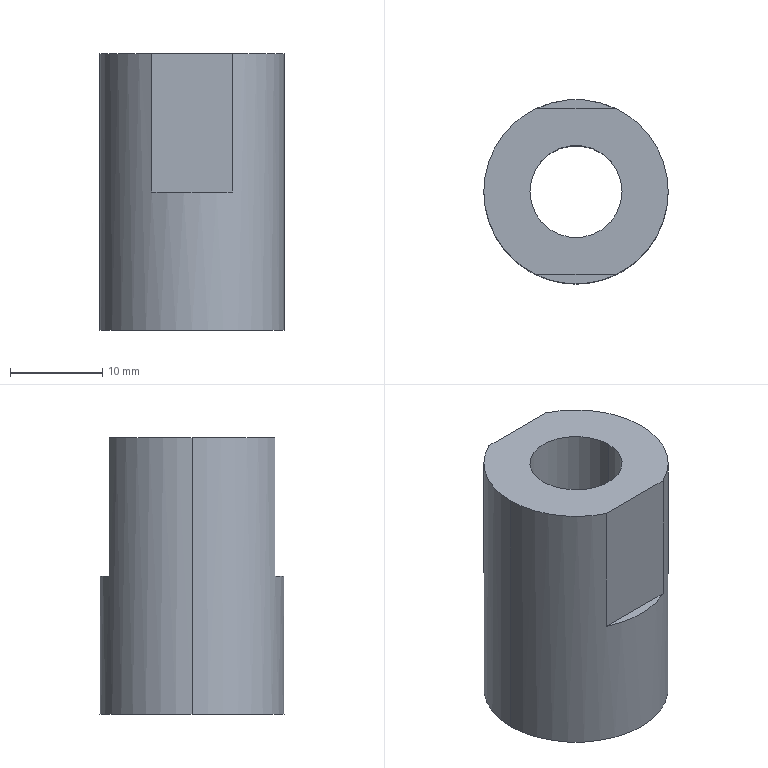Part | STEP file | Cylinder joint | 1 solid | 10 faces | box 20 x 20 x 30 mm | volume 6892 mm3 | plane 6 | cylinder 4 | commonest cylinder face diameters 10 x2 20 x2
STEP:
#1=CARTESIAN_POINT('',(0.,0.,0.));
#2=DIRECTION('',(0.,0.,1.));
#3=DIRECTION('',(1.,0.,0.));
#4=AXIS2_PLACEMENT_3D('',#1,#2,#3);
#5=CARTESIAN_POINT('',(4.359,9.,30.));
#6=VERTEX_POINT('',#5);
#7=CARTESIAN_POINT('',(10.,0.,30.));
#8=VERTEX_POINT('',#7);
#9=CARTESIAN_POINT('',(0.,0.,30.));
#10=DIRECTION('',(0.,0.,-1.));
#11=DIRECTION('',(-1.,0.,0.));
#12=AXIS2_PLACEMENT_3D('',#9,#10,#11);
#13=CIRCLE('',#12,10.);
#14=CARTESIAN_POINT('',(0.,0.,30.));
#15=DIRECTION('',(0.,0.,-1.));
#16=DIRECTION('',(-1.,0.,0.));
#17=AXIS2_PLACEMENT_3D('',#14,#15,#16);
#18=CYLINDRICAL_SURFACE('',#17,10.);
#19=CARTESIAN_POINT('',(0.,0.));
#20=DIRECTION('',(1.,0.));
#21=VECTOR('',#20,1.);
#22=LINE('',#19,#21);
#23=(GEOMETRIC_REPRESENTATION_CONTEXT(2)PARAMETRIC_REPRESENTATION_CONTEXT()REPRESENTATION_CONTEXT('',''));
#24=DEFINITIONAL_REPRESENTATION('',(#22),#23);
#25=PCURVE('',#18,#24);
#26=CARTESIAN_POINT('',(0.,0.,30.));
#27=DIRECTION('',(0.,0.,1.));
#28=DIRECTION('',(1.,0.,0.));
#29=AXIS2_PLACEMENT_3D('',#26,#27,#28);
#30=PLANE('',#29);
#31=CARTESIAN_POINT('',(-10.,0.));
#32=CARTESIAN_POINT('',(-10.,17.321));
#33=CARTESIAN_POINT('',(5.,8.66));
#34=CARTESIAN_POINT('',(20.,0.));
#35=CARTESIAN_POINT('',(5.,-8.66));
#36=CARTESIAN_POINT('',(-10.,-17.321));
#37=CARTESIAN_POINT('',(-10.,0.));
#38=(BOUNDED_CURVE()B_SPLINE_CURVE(2,(#31,#32,#33,#34,#35,#36,#37),.UNSPECIFIED.,.T.,.F.)B_SPLINE_CURVE_WITH_KNOTS((1,2,2,2,2,1),(-2.094,0.,2.094,4.189,6.283,8.378),.UNSPECIFIED.)CURVE()GEOMETRIC_REPRESENTATION_ITEM()RATIONAL_B_SPLINE_CURVE((1.,0.5,1.,0.5,1.,0.5,1.))REPRESENTATION_ITEM(''));
#39=(GEOMETRIC_REPRESENTATION_CONTEXT(2)PARAMETRIC_REPRESENTATION_CONTEXT()REPRESENTATION_CONTEXT('',''));
#40=DEFINITIONAL_REPRESENTATION('',(#38),#39);
#41=PCURVE('',#30,#40);
#42=SURFACE_CURVE('',#13,(#25,#41),.PCURVE_S1.);
#43=EDGE_CURVE('',#6,#8,#42,.T.);
#44=ORIENTED_EDGE('',*,*,#43,.T.);
#45=CARTESIAN_POINT('',(10.,0.,0.));
#46=VERTEX_POINT('',#45);
#47=CARTESIAN_POINT('',(10.,0.,30.));
#48=DIRECTION('',(0.,0.,-1.));
#49=VECTOR('',#48,1.);
#50=LINE('',#47,#49);
#51=CARTESIAN_POINT('',(3.142,0.));
#52=DIRECTION('',(0.,1.));
#53=VECTOR('',#52,1.);
#54=LINE('',#51,#53);
#55=(GEOMETRIC_REPRESENTATION_CONTEXT(2)PARAMETRIC_REPRESENTATION_CONTEXT()REPRESENTATION_CONTEXT('',''));
#56=DEFINITIONAL_REPRESENTATION('',(#54),#55);
#57=PCURVE('',#18,#56);
#58=CARTESIAN_POINT('',(0.,0.,30.));
#59=DIRECTION('',(0.,0.,-1.));
#60=DIRECTION('',(-1.,0.,0.));
#61=AXIS2_PLACEMENT_3D('',#58,#59,#60);
#62=CYLINDRICAL_SURFACE('',#61,10.);
#63=CARTESIAN_POINT('',(3.142,0.));
#64=DIRECTION('',(0.,1.));
#65=VECTOR('',#64,1.);
#66=LINE('',#63,#65);
#67=(GEOMETRIC_REPRESENTATION_CONTEXT(2)PARAMETRIC_REPRESENTATION_CONTEXT()REPRESENTATION_CONTEXT('',''));
#68=DEFINITIONAL_REPRESENTATION('',(#66),#67);
#69=PCURVE('',#62,#68);
#70=SURFACE_CURVE('',#50,(#57,#69),.PCURVE_S1.);
#71=EDGE_CURVE('',#8,#46,#70,.T.);
#72=ORIENTED_EDGE('',*,*,#71,.T.);
#73=CARTESIAN_POINT('',(-10.,0.,0.));
#74=VERTEX_POINT('',#73);
#75=CARTESIAN_POINT('',(0.,0.,0.));
#76=DIRECTION('',(0.,0.,1.));
#77=DIRECTION('',(-1.,0.,0.));
#78=AXIS2_PLACEMENT_3D('',#75,#76,#77);
#79=CIRCLE('',#78,10.);
#80=CARTESIAN_POINT('',(6.283,30.));
#81=DIRECTION('',(-1.,0.));
#82=VECTOR('',#81,1.);
#83=LINE('',#80,#82);
#84=(GEOMETRIC_REPRESENTATION_CONTEXT(2)PARAMETRIC_REPRESENTATION_CONTEXT()REPRESENTATION_CONTEXT('',''));
#85=DEFINITIONAL_REPRESENTATION('',(#83),#84);
#86=PCURVE('',#18,#85);
#87=CARTESIAN_POINT('',(0.,0.,0.));
#88=DIRECTION('',(0.,0.,1.));
#89=DIRECTION('',(1.,0.,0.));
#90=AXIS2_PLACEMENT_3D('',#87,#88,#89);
#91=PLANE('',#90);
#92=CARTESIAN_POINT('',(0.,0.));
#93=DIRECTION('',(-1.,0.));
#94=AXIS2_PLACEMENT_2D('',#92,#93);
#95=CIRCLE('',#94,10.);
#96=(GEOMETRIC_REPRESENTATION_CONTEXT(2)PARAMETRIC_REPRESENTATION_CONTEXT()REPRESENTATION_CONTEXT('',''));
#97=DEFINITIONAL_REPRESENTATION('',(#95),#96);
#98=PCURVE('',#91,#97);
#99=SURFACE_CURVE('',#79,(#86,#98),.PCURVE_S1.);
#100=EDGE_CURVE('',#46,#74,#99,.T.);
#101=ORIENTED_EDGE('',*,*,#100,.T.);
#102=CARTESIAN_POINT('',(-10.,0.,30.));
#103=VERTEX_POINT('',#102);
#104=CARTESIAN_POINT('',(-10.,0.,30.));
#105=DIRECTION('',(0.,0.,-1.));
#106=VECTOR('',#105,1.);
#107=LINE('',#104,#106);
#108=CARTESIAN_POINT('',(0.,0.));
#109=DIRECTION('',(0.,1.));
#110=VECTOR('',#109,1.);
#111=LINE('',#108,#110);
#112=(GEOMETRIC_REPRESENTATION_CONTEXT(2)PARAMETRIC_REPRESENTATION_CONTEXT()REPRESENTATION_CONTEXT('',''));
#113=DEFINITIONAL_REPRESENTATION('',(#111),#112);
#114=PCURVE('',#18,#113);
#115=CARTESIAN_POINT('',(6.283,0.));
#116=DIRECTION('',(0.,1.));
#117=VECTOR('',#116,1.);
#118=LINE('',#115,#117);
#119=(GEOMETRIC_REPRESENTATION_CONTEXT(2)PARAMETRIC_REPRESENTATION_CONTEXT()REPRESENTATION_CONTEXT('',''));
#120=DEFINITIONAL_REPRESENTATION('',(#118),#119);
#121=PCURVE('',#62,#120);
#122=SURFACE_CURVE('',#107,(#114,#121),.PCURVE_S1.);
#123=EDGE_CURVE('',#103,#74,#122,.T.);
#124=ORIENTED_EDGE('',*,*,#123,.F.);
#125=CARTESIAN_POINT('',(-4.359,9.,30.));
#126=VERTEX_POINT('',#125);
#127=CARTESIAN_POINT('',(0.,0.,30.));
#128=DIRECTION('',(0.,0.,-1.));
#129=DIRECTION('',(-1.,0.,0.));
#130=AXIS2_PLACEMENT_3D('',#127,#128,#129);
#131=CIRCLE('',#130,10.);
#132=CARTESIAN_POINT('',(0.,0.));
#133=DIRECTION('',(1.,0.));
#134=VECTOR('',#133,1.);
#135=LINE('',#132,#134);
#136=(GEOMETRIC_REPRESENTATION_CONTEXT(2)PARAMETRIC_REPRESENTATION_CONTEXT()REPRESENTATION_CONTEXT('',''));
#137=DEFINITIONAL_REPRESENTATION('',(#135),#136);
#138=PCURVE('',#18,#137);
#139=CARTESIAN_POINT('',(-10.,0.));
#140=CARTESIAN_POINT('',(-10.,17.321));
#141=CARTESIAN_POINT('',(5.,8.66));
#142=CARTESIAN_POINT('',(20.,0.));
#143=CARTESIAN_POINT('',(5.,-8.66));
#144=CARTESIAN_POINT('',(-10.,-17.321));
#145=CARTESIAN_POINT('',(-10.,0.));
#146=(BOUNDED_CURVE()B_SPLINE_CURVE(2,(#139,#140,#141,#142,#143,#144,#145),.UNSPECIFIED.,.T.,.F.)B_SPLINE_CURVE_WITH_KNOTS((1,2,2,2,2,1),(-2.094,0.,2.094,4.189,6.283,8.378),.UNSPECIFIED.)CURVE()GEOMETRIC_REPRESENTATION_ITEM()RATIONAL_B_SPLINE_CURVE((1.,0.5,1.,0.5,1.,0.5,1.))REPRESENTATION_ITEM(''));
#147=(GEOMETRIC_REPRESENTATION_CONTEXT(2)PARAMETRIC_REPRESENTATION_CONTEXT()REPRESENTATION_CONTEXT('',''));
#148=DEFINITIONAL_REPRESENTATION('',(#146),#147);
#149=PCURVE('',#30,#148);
#150=SURFACE_CURVE('',#131,(#138,#149),.PCURVE_S1.);
#151=EDGE_CURVE('',#103,#126,#150,.T.);
#152=ORIENTED_EDGE('',*,*,#151,.T.);
#153=CARTESIAN_POINT('',(-4.359,9.,15.));
#154=VERTEX_POINT('',#153);
#155=CARTESIAN_POINT('',(-4.359,9.,30.));
#156=DIRECTION('',(0.,0.,-1.));
#157=VECTOR('',#156,1.);
#158=LINE('',#155,#157);
#159=CARTESIAN_POINT('',(1.12,0.));
#160=DIRECTION('',(0.,1.));
#161=VECTOR('',#160,1.);
#162=LINE('',#159,#161);
#163=(GEOMETRIC_REPRESENTATION_CONTEXT(2)PARAMETRIC_REPRESENTATION_CONTEXT()REPRESENTATION_CONTEXT('',''));
#164=DEFINITIONAL_REPRESENTATION('',(#162),#163);
#165=PCURVE('',#18,#164);
#166=CARTESIAN_POINT('',(-4.359,9.,15.));
#167=DIRECTION('',(0.,-1.,0.));
#168=DIRECTION('',(0.,0.,-1.));
#169=AXIS2_PLACEMENT_3D('',#166,#167,#168);
#170=PLANE('',#169);
#171=CARTESIAN_POINT('',(-15.,0.));
#172=DIRECTION('',(1.,0.));
#173=VECTOR('',#172,1.);
#174=LINE('',#171,#173);
#175=(GEOMETRIC_REPRESENTATION_CONTEXT(2)PARAMETRIC_REPRESENTATION_CONTEXT()REPRESENTATION_CONTEXT('',''));
#176=DEFINITIONAL_REPRESENTATION('',(#174),#175);
#177=PCURVE('',#170,#176);
#178=SURFACE_CURVE('',#158,(#165,#177),.PCURVE_S1.);
#179=EDGE_CURVE('',#126,#154,#178,.T.);
#180=ORIENTED_EDGE('',*,*,#179,.T.);
#181=CARTESIAN_POINT('',(4.359,9.,15.));
#182=VERTEX_POINT('',#181);
#183=CARTESIAN_POINT('',(0.,0.,15.));
#184=DIRECTION('',(0.,0.,-1.));
#185=DIRECTION('',(-1.,0.,0.));
#186=AXIS2_PLACEMENT_3D('',#183,#184,#185);
#187=CIRCLE('',#186,10.);
#188=CARTESIAN_POINT('',(0.,15.));
#189=DIRECTION('',(1.,0.));
#190=VECTOR('',#189,1.);
#191=LINE('',#188,#190);
#192=(GEOMETRIC_REPRESENTATION_CONTEXT(2)PARAMETRIC_REPRESENTATION_CONTEXT()REPRESENTATION_CONTEXT('',''));
#193=DEFINITIONAL_REPRESENTATION('',(#191),#192);
#194=PCURVE('',#18,#193);
#195=CARTESIAN_POINT('',(0.,0.,15.));
#196=DIRECTION('',(0.,0.,1.));
#197=DIRECTION('',(1.,0.,0.));
#198=AXIS2_PLACEMENT_3D('',#195,#196,#197);
#199=PLANE('',#198);
#200=CARTESIAN_POINT('',(-10.,0.));
#201=CARTESIAN_POINT('',(-10.,17.321));
#202=CARTESIAN_POINT('',(5.,8.66));
#203=CARTESIAN_POINT('',(20.,0.));
#204=CARTESIAN_POINT('',(5.,-8.66));
#205=CARTESIAN_POINT('',(-10.,-17.321));
#206=CARTESIAN_POINT('',(-10.,0.));
#207=(BOUNDED_CURVE()B_SPLINE_CURVE(2,(#200,#201,#202,#203,#204,#205,#206),.UNSPECIFIED.,.T.,.F.)B_SPLINE_CURVE_WITH_KNOTS((1,2,2,2,2,1),(-2.094,0.,2.094,4.189,6.283,8.378),.UNSPECIFIED.)CURVE()GEOMETRIC_REPRESENTATION_ITEM()RATIONAL_B_SPLINE_CURVE((1.,0.5,1.,0.5,1.,0.5,1.))REPRESENTATION_ITEM(''));
#208=(GEOMETRIC_REPRESENTATION_CONTEXT(2)PARAMETRIC_REPRESENTATION_CONTEXT()REPRESENTATION_CONTEXT('',''));
#209=DEFINITIONAL_REPRESENTATION('',(#207),#208);
#210=PCURVE('',#199,#209);
#211=SURFACE_CURVE('',#187,(#194,#210),.PCURVE_S1.);
#212=EDGE_CURVE('',#154,#182,#211,.T.);
#213=ORIENTED_EDGE('',*,*,#212,.T.);
#214=CARTESIAN_POINT('',(4.359,9.,30.));
#215=DIRECTION('',(0.,0.,1.));
#216=VECTOR('',#215,1.);
#217=LINE('',#214,#216);
#218=CARTESIAN_POINT('',(2.022,0.));
#219=DIRECTION('',(0.,-1.));
#220=VECTOR('',#219,1.);
#221=LINE('',#218,#220);
#222=(GEOMETRIC_REPRESENTATION_CONTEXT(2)PARAMETRIC_REPRESENTATION_CONTEXT()REPRESENTATION_CONTEXT('',''));
#223=DEFINITIONAL_REPRESENTATION('',(#221),#222);
#224=PCURVE('',#18,#223);
#225=CARTESIAN_POINT('',(-15.,8.718));
#226=DIRECTION('',(-1.,0.));
#227=VECTOR('',#226,1.);
#228=LINE('',#225,#227);
#229=(GEOMETRIC_REPRESENTATION_CONTEXT(2)PARAMETRIC_REPRESENTATION_CONTEXT()REPRESENTATION_CONTEXT('',''));
#230=DEFINITIONAL_REPRESENTATION('',(#228),#229);
#231=PCURVE('',#170,#230);
#232=SURFACE_CURVE('',#217,(#224,#231),.PCURVE_S1.);
#233=EDGE_CURVE('',#182,#6,#232,.T.);
#234=ORIENTED_EDGE('',*,*,#233,.T.);
#235=EDGE_LOOP('',(#44,#72,#101,#124,#152,#180,#213,#234));
#236=FACE_BOUND('',#235,.T.);
#237=ADVANCED_FACE('',(#236),#18,.T.);
#238=CARTESIAN_POINT('',(-5.,0.,30.));
#239=VERTEX_POINT('',#238);
#240=CARTESIAN_POINT('',(-5.,0.,0.));
#241=VERTEX_POINT('',#240);
#242=CARTESIAN_POINT('',(-5.,0.,30.));
#243=DIRECTION('',(0.,0.,-1.));
#244=VECTOR('',#243,1.);
#245=LINE('',#242,#244);
#246=CARTESIAN_POINT('',(0.,0.,30.));
#247=DIRECTION('',(0.,0.,-1.));
#248=DIRECTION('',(-1.,0.,0.));
#249=AXIS2_PLACEMENT_3D('',#246,#247,#248);
#250=CYLINDRICAL_SURFACE('',#249,5.);
#251=CARTESIAN_POINT('',(6.283,0.));
#252=DIRECTION('',(0.,1.));
#253=VECTOR('',#252,1.);
#254=LINE('',#251,#253);
#255=(GEOMETRIC_REPRESENTATION_CONTEXT(2)PARAMETRIC_REPRESENTATION_CONTEXT()REPRESENTATION_CONTEXT('',''));
#256=DEFINITIONAL_REPRESENTATION('',(#254),#255);
#257=PCURVE('',#250,#256);
#258=CARTESIAN_POINT('',(0.,0.,30.));
#259=DIRECTION('',(0.,0.,-1.));
#260=DIRECTION('',(-1.,0.,0.));
#261=AXIS2_PLACEMENT_3D('',#258,#259,#260);
#262=CYLINDRICAL_SURFACE('',#261,5.);
#263=CARTESIAN_POINT('',(0.,0.));
#264=DIRECTION('',(0.,1.));
#265=VECTOR('',#264,1.);
#266=LINE('',#263,#265);
#267=(GEOMETRIC_REPRESENTATION_CONTEXT(2)PARAMETRIC_REPRESENTATION_CONTEXT()REPRESENTATION_CONTEXT('',''));
#268=DEFINITIONAL_REPRESENTATION('',(#266),#267);
#269=PCURVE('',#262,#268);
#270=SURFACE_CURVE('',#245,(#257,#269),.PCURVE_S1.);
#271=EDGE_CURVE('',#239,#241,#270,.T.);
#272=ORIENTED_EDGE('',*,*,#271,.T.);
#273=CARTESIAN_POINT('',(5.,0.,0.));
#274=VERTEX_POINT('',#273);
#275=CARTESIAN_POINT('',(0.,0.,0.));
#276=DIRECTION('',(0.,0.,-1.));
#277=DIRECTION('',(-1.,0.,0.));
#278=AXIS2_PLACEMENT_3D('',#275,#276,#277);
#279=CIRCLE('',#278,5.);
#280=CARTESIAN_POINT('',(0.,30.));
#281=DIRECTION('',(1.,0.));
#282=VECTOR('',#281,1.);
#283=LINE('',#280,#282);
#284=(GEOMETRIC_REPRESENTATION_CONTEXT(2)PARAMETRIC_REPRESENTATION_CONTEXT()REPRESENTATION_CONTEXT('',''));
#285=DEFINITIONAL_REPRESENTATION('',(#283),#284);
#286=PCURVE('',#250,#285);
#287=CARTESIAN_POINT('',(-5.,0.));
#288=CARTESIAN_POINT('',(-5.,8.66));
#289=CARTESIAN_POINT('',(2.5,4.33));
#290=CARTESIAN_POINT('',(10.,0.));
#291=CARTESIAN_POINT('',(2.5,-4.33));
#292=CARTESIAN_POINT('',(-5.,-8.66));
#293=CARTESIAN_POINT('',(-5.,0.));
#294=(BOUNDED_CURVE()B_SPLINE_CURVE(2,(#287,#288,#289,#290,#291,#292,#293),.UNSPECIFIED.,.T.,.F.)B_SPLINE_CURVE_WITH_KNOTS((1,2,2,2,2,1),(-2.094,0.,2.094,4.189,6.283,8.378),.UNSPECIFIED.)CURVE()GEOMETRIC_REPRESENTATION_ITEM()RATIONAL_B_SPLINE_CURVE((1.,0.5,1.,0.5,1.,0.5,1.))REPRESENTATION_ITEM(''));
#295=(GEOMETRIC_REPRESENTATION_CONTEXT(2)PARAMETRIC_REPRESENTATION_CONTEXT()REPRESENTATION_CONTEXT('',''));
#296=DEFINITIONAL_REPRESENTATION('',(#294),#295);
#297=PCURVE('',#91,#296);
#298=SURFACE_CURVE('',#279,(#286,#297),.PCURVE_S1.);
#299=EDGE_CURVE('',#274,#241,#298,.T.);
#300=ORIENTED_EDGE('',*,*,#299,.F.);
#301=CARTESIAN_POINT('',(5.,0.,30.));
#302=VERTEX_POINT('',#301);
#303=CARTESIAN_POINT('',(5.,0.,30.));
#304=DIRECTION('',(0.,0.,-1.));
#305=VECTOR('',#304,1.);
#306=LINE('',#303,#305);
#307=CARTESIAN_POINT('',(3.142,0.));
#308=DIRECTION('',(0.,1.));
#309=VECTOR('',#308,1.);
#310=LINE('',#307,#309);
#311=(GEOMETRIC_REPRESENTATION_CONTEXT(2)PARAMETRIC_REPRESENTATION_CONTEXT()REPRESENTATION_CONTEXT('',''));
#312=DEFINITIONAL_REPRESENTATION('',(#310),#311);
#313=PCURVE('',#250,#312);
#314=CARTESIAN_POINT('',(3.142,0.));
#315=DIRECTION('',(0.,1.));
#316=VECTOR('',#315,1.);
#317=LINE('',#314,#316);
#318=(GEOMETRIC_REPRESENTATION_CONTEXT(2)PARAMETRIC_REPRESENTATION_CONTEXT()REPRESENTATION_CONTEXT('',''));
#319=DEFINITIONAL_REPRESENTATION('',(#317),#318);
#320=PCURVE('',#262,#319);
#321=SURFACE_CURVE('',#306,(#313,#320),.PCURVE_S1.);
#322=EDGE_CURVE('',#302,#274,#321,.T.);
#323=ORIENTED_EDGE('',*,*,#322,.F.);
#324=CARTESIAN_POINT('',(0.,0.,30.));
#325=DIRECTION('',(0.,0.,-1.));
#326=DIRECTION('',(-1.,0.,0.));
#327=AXIS2_PLACEMENT_3D('',#324,#325,#326);
#328=CIRCLE('',#327,5.);
#329=CARTESIAN_POINT('',(0.,0.));
#330=DIRECTION('',(1.,0.));
#331=VECTOR('',#330,1.);
#332=LINE('',#329,#331);
#333=(GEOMETRIC_REPRESENTATION_CONTEXT(2)PARAMETRIC_REPRESENTATION_CONTEXT()REPRESENTATION_CONTEXT('',''));
#334=DEFINITIONAL_REPRESENTATION('',(#332),#333);
#335=PCURVE('',#250,#334);
#336=CARTESIAN_POINT('',(-5.,0.));
#337=CARTESIAN_POINT('',(-5.,8.66));
#338=CARTESIAN_POINT('',(2.5,4.33));
#339=CARTESIAN_POINT('',(10.,0.));
#340=CARTESIAN_POINT('',(2.5,-4.33));
#341=CARTESIAN_POINT('',(-5.,-8.66));
#342=CARTESIAN_POINT('',(-5.,0.));
#343=(BOUNDED_CURVE()B_SPLINE_CURVE(2,(#336,#337,#338,#339,#340,#341,#342),.UNSPECIFIED.,.T.,.F.)B_SPLINE_CURVE_WITH_KNOTS((1,2,2,2,2,1),(-2.094,0.,2.094,4.189,6.283,8.378),.UNSPECIFIED.)CURVE()GEOMETRIC_REPRESENTATION_ITEM()RATIONAL_B_SPLINE_CURVE((1.,0.5,1.,0.5,1.,0.5,1.))REPRESENTATION_ITEM(''));
#344=(GEOMETRIC_REPRESENTATION_CONTEXT(2)PARAMETRIC_REPRESENTATION_CONTEXT()REPRESENTATION_CONTEXT('',''));
#345=DEFINITIONAL_REPRESENTATION('',(#343),#344);
#346=PCURVE('',#30,#345);
#347=SURFACE_CURVE('',#328,(#335,#346),.PCURVE_S1.);
#348=EDGE_CURVE('',#302,#239,#347,.T.);
#349=ORIENTED_EDGE('',*,*,#348,.T.);
#350=EDGE_LOOP('',(#272,#300,#323,#349));
#351=FACE_BOUND('',#350,.F.);
#352=ADVANCED_FACE('',(#351),#250,.F.);
#353=ORIENTED_EDGE('',*,*,#71,.F.);
#354=CARTESIAN_POINT('',(4.359,-9.,30.));
#355=VERTEX_POINT('',#354);
#356=CARTESIAN_POINT('',(0.,0.,30.));
#357=DIRECTION('',(0.,0.,-1.));
#358=DIRECTION('',(-1.,0.,0.));
#359=AXIS2_PLACEMENT_3D('',#356,#357,#358);
#360=CIRCLE('',#359,10.);
#361=CARTESIAN_POINT('',(0.,0.));
#362=DIRECTION('',(1.,0.));
#363=VECTOR('',#362,1.);
#364=LINE('',#361,#363);
#365=(GEOMETRIC_REPRESENTATION_CONTEXT(2)PARAMETRIC_REPRESENTATION_CONTEXT()REPRESENTATION_CONTEXT('',''));
#366=DEFINITIONAL_REPRESENTATION('',(#364),#365);
#367=PCURVE('',#62,#366);
#368=CARTESIAN_POINT('',(-10.,0.));
#369=CARTESIAN_POINT('',(-10.,17.321));
#370=CARTESIAN_POINT('',(5.,8.66));
#371=CARTESIAN_POINT('',(20.,0.));
#372=CARTESIAN_POINT('',(5.,-8.66));
#373=CARTESIAN_POINT('',(-10.,-17.321));
#374=CARTESIAN_POINT('',(-10.,0.));
#375=(BOUNDED_CURVE()B_SPLINE_CURVE(2,(#368,#369,#370,#371,#372,#373,#374),.UNSPECIFIED.,.T.,.F.)B_SPLINE_CURVE_WITH_KNOTS((1,2,2,2,2,1),(-2.094,0.,2.094,4.189,6.283,8.378),.UNSPECIFIED.)CURVE()GEOMETRIC_REPRESENTATION_ITEM()RATIONAL_B_SPLINE_CURVE((1.,0.5,1.,0.5,1.,0.5,1.))REPRESENTATION_ITEM(''));
#376=(GEOMETRIC_REPRESENTATION_CONTEXT(2)PARAMETRIC_REPRESENTATION_CONTEXT()REPRESENTATION_CONTEXT('',''));
#377=DEFINITIONAL_REPRESENTATION('',(#375),#376);
#378=PCURVE('',#30,#377);
#379=SURFACE_CURVE('',#360,(#367,#378),.PCURVE_S1.);
#380=EDGE_CURVE('',#8,#355,#379,.T.);
#381=ORIENTED_EDGE('',*,*,#380,.T.);
#382=CARTESIAN_POINT('',(4.359,-9.,15.));
#383=VERTEX_POINT('',#382);
#384=CARTESIAN_POINT('',(4.359,-9.,30.));
#385=DIRECTION('',(0.,0.,-1.));
#386=VECTOR('',#385,1.);
#387=LINE('',#384,#386);
#388=CARTESIAN_POINT('',(4.261,0.));
#389=DIRECTION('',(0.,1.));
#390=VECTOR('',#389,1.);
#391=LINE('',#388,#390);
#392=(GEOMETRIC_REPRESENTATION_CONTEXT(2)PARAMETRIC_REPRESENTATION_CONTEXT()REPRESENTATION_CONTEXT('',''));
#393=DEFINITIONAL_REPRESENTATION('',(#391),#392);
#394=PCURVE('',#62,#393);
#395=CARTESIAN_POINT('',(-4.359,-9.,15.));
#396=DIRECTION('',(0.,1.,0.));
#397=DIRECTION('',(0.,0.,1.));
#398=AXIS2_PLACEMENT_3D('',#395,#396,#397);
#399=PLANE('',#398);
#400=CARTESIAN_POINT('',(15.,8.718));
#401=DIRECTION('',(-1.,0.));
#402=VECTOR('',#401,1.);
#403=LINE('',#400,#402);
#404=(GEOMETRIC_REPRESENTATION_CONTEXT(2)PARAMETRIC_REPRESENTATION_CONTEXT()REPRESENTATION_CONTEXT('',''));
#405=DEFINITIONAL_REPRESENTATION('',(#403),#404);
#406=PCURVE('',#399,#405);
#407=SURFACE_CURVE('',#387,(#394,#406),.PCURVE_S1.);
#408=EDGE_CURVE('',#355,#383,#407,.T.);
#409=ORIENTED_EDGE('',*,*,#408,.T.);
#410=CARTESIAN_POINT('',(-4.359,-9.,15.));
#411=VERTEX_POINT('',#410);
#412=CARTESIAN_POINT('',(0.,0.,15.));
#413=DIRECTION('',(0.,0.,-1.));
#414=DIRECTION('',(-1.,0.,0.));
#415=AXIS2_PLACEMENT_3D('',#412,#413,#414);
#416=CIRCLE('',#415,10.);
#417=CARTESIAN_POINT('',(0.,15.));
#418=DIRECTION('',(1.,0.));
#419=VECTOR('',#418,1.);
#420=LINE('',#417,#419);
#421=(GEOMETRIC_REPRESENTATION_CONTEXT(2)PARAMETRIC_REPRESENTATION_CONTEXT()REPRESENTATION_CONTEXT('',''));
#422=DEFINITIONAL_REPRESENTATION('',(#420),#421);
#423=PCURVE('',#62,#422);
#424=CARTESIAN_POINT('',(0.,0.,15.));
#425=DIRECTION('',(0.,0.,1.));
#426=DIRECTION('',(1.,0.,0.));
#427=AXIS2_PLACEMENT_3D('',#424,#425,#426);
#428=PLANE('',#427);
#429=CARTESIAN_POINT('',(-10.,0.));
#430=CARTESIAN_POINT('',(-10.,17.321));
#431=CARTESIAN_POINT('',(5.,8.66));
#432=CARTESIAN_POINT('',(20.,0.));
#433=CARTESIAN_POINT('',(5.,-8.66));
#434=CARTESIAN_POINT('',(-10.,-17.321));
#435=CARTESIAN_POINT('',(-10.,0.));
#436=(BOUNDED_CURVE()B_SPLINE_CURVE(2,(#429,#430,#431,#432,#433,#434,#435),.UNSPECIFIED.,.T.,.F.)B_SPLINE_CURVE_WITH_KNOTS((1,2,2,2,2,1),(-2.094,0.,2.094,4.189,6.283,8.378),.UNSPECIFIED.)CURVE()GEOMETRIC_REPRESENTATION_ITEM()RATIONAL_B_SPLINE_CURVE((1.,0.5,1.,0.5,1.,0.5,1.))REPRESENTATION_ITEM(''));
#437=(GEOMETRIC_REPRESENTATION_CONTEXT(2)PARAMETRIC_REPRESENTATION_CONTEXT()REPRESENTATION_CONTEXT('',''));
#438=DEFINITIONAL_REPRESENTATION('',(#436),#437);
#439=PCURVE('',#428,#438);
#440=SURFACE_CURVE('',#416,(#423,#439),.PCURVE_S1.);
#441=EDGE_CURVE('',#383,#411,#440,.T.);
#442=ORIENTED_EDGE('',*,*,#441,.T.);
#443=CARTESIAN_POINT('',(-4.359,-9.,30.));
#444=VERTEX_POINT('',#443);
#445=CARTESIAN_POINT('',(-4.359,-9.,30.));
#446=DIRECTION('',(0.,0.,1.));
#447=VECTOR('',#446,1.);
#448=LINE('',#445,#447);
#449=CARTESIAN_POINT('',(5.163,0.));
#450=DIRECTION('',(0.,-1.));
#451=VECTOR('',#450,1.);
#452=LINE('',#449,#451);
#453=(GEOMETRIC_REPRESENTATION_CONTEXT(2)PARAMETRIC_REPRESENTATION_CONTEXT()REPRESENTATION_CONTEXT('',''));
#454=DEFINITIONAL_REPRESENTATION('',(#452),#453);
#455=PCURVE('',#62,#454);
#456=CARTESIAN_POINT('',(15.,0.));
#457=DIRECTION('',(1.,0.));
#458=VECTOR('',#457,1.);
#459=LINE('',#456,#458);
#460=(GEOMETRIC_REPRESENTATION_CONTEXT(2)PARAMETRIC_REPRESENTATION_CONTEXT()REPRESENTATION_CONTEXT('',''));
#461=DEFINITIONAL_REPRESENTATION('',(#459),#460);
#462=PCURVE('',#399,#461);
#463=SURFACE_CURVE('',#448,(#455,#462),.PCURVE_S1.);
#464=EDGE_CURVE('',#411,#444,#463,.T.);
#465=ORIENTED_EDGE('',*,*,#464,.T.);
#466=CARTESIAN_POINT('',(0.,0.,30.));
#467=DIRECTION('',(0.,0.,-1.));
#468=DIRECTION('',(-1.,0.,0.));
#469=AXIS2_PLACEMENT_3D('',#466,#467,#468);
#470=CIRCLE('',#469,10.);
#471=CARTESIAN_POINT('',(0.,0.));
#472=DIRECTION('',(1.,0.));
#473=VECTOR('',#472,1.);
#474=LINE('',#471,#473);
#475=(GEOMETRIC_REPRESENTATION_CONTEXT(2)PARAMETRIC_REPRESENTATION_CONTEXT()REPRESENTATION_CONTEXT('',''));
#476=DEFINITIONAL_REPRESENTATION('',(#474),#475);
#477=PCURVE('',#62,#476);
#478=CARTESIAN_POINT('',(-10.,0.));
#479=CARTESIAN_POINT('',(-10.,17.321));
#480=CARTESIAN_POINT('',(5.,8.66));
#481=CARTESIAN_POINT('',(20.,0.));
#482=CARTESIAN_POINT('',(5.,-8.66));
#483=CARTESIAN_POINT('',(-10.,-17.321));
#484=CARTESIAN_POINT('',(-10.,0.));
#485=(BOUNDED_CURVE()B_SPLINE_CURVE(2,(#478,#479,#480,#481,#482,#483,#484),.UNSPECIFIED.,.T.,.F.)B_SPLINE_CURVE_WITH_KNOTS((1,2,2,2,2,1),(-2.094,0.,2.094,4.189,6.283,8.378),.UNSPECIFIED.)CURVE()GEOMETRIC_REPRESENTATION_ITEM()RATIONAL_B_SPLINE_CURVE((1.,0.5,1.,0.5,1.,0.5,1.))REPRESENTATION_ITEM(''));
#486=(GEOMETRIC_REPRESENTATION_CONTEXT(2)PARAMETRIC_REPRESENTATION_CONTEXT()REPRESENTATION_CONTEXT('',''));
#487=DEFINITIONAL_REPRESENTATION('',(#485),#486);
#488=PCURVE('',#30,#487);
#489=SURFACE_CURVE('',#470,(#477,#488),.PCURVE_S1.);
#490=EDGE_CURVE('',#444,#103,#489,.T.);
#491=ORIENTED_EDGE('',*,*,#490,.T.);
#492=ORIENTED_EDGE('',*,*,#123,.T.);
#493=CARTESIAN_POINT('',(0.,0.,0.));
#494=DIRECTION('',(0.,0.,1.));
#495=DIRECTION('',(-1.,0.,0.));
#496=AXIS2_PLACEMENT_3D('',#493,#494,#495);
#497=CIRCLE('',#496,10.);
#498=CARTESIAN_POINT('',(6.283,30.));
#499=DIRECTION('',(-1.,0.));
#500=VECTOR('',#499,1.);
#501=LINE('',#498,#500);
#502=(GEOMETRIC_REPRESENTATION_CONTEXT(2)PARAMETRIC_REPRESENTATION_CONTEXT()REPRESENTATION_CONTEXT('',''));
#503=DEFINITIONAL_REPRESENTATION('',(#501),#502);
#504=PCURVE('',#62,#503);
#505=CARTESIAN_POINT('',(0.,0.));
#506=DIRECTION('',(-1.,0.));
#507=AXIS2_PLACEMENT_2D('',#505,#506);
#508=CIRCLE('',#507,10.);
#509=(GEOMETRIC_REPRESENTATION_CONTEXT(2)PARAMETRIC_REPRESENTATION_CONTEXT()REPRESENTATION_CONTEXT('',''));
#510=DEFINITIONAL_REPRESENTATION('',(#508),#509);
#511=PCURVE('',#91,#510);
#512=SURFACE_CURVE('',#497,(#504,#511),.PCURVE_S1.);
#513=EDGE_CURVE('',#74,#46,#512,.T.);
#514=ORIENTED_EDGE('',*,*,#513,.T.);
#515=EDGE_LOOP('',(#353,#381,#409,#442,#465,#491,#492,#514));
#516=FACE_BOUND('',#515,.T.);
#517=ADVANCED_FACE('',(#516),#62,.T.);
#518=ORIENTED_EDGE('',*,*,#233,.F.);
#519=CARTESIAN_POINT('',(-4.359,9.,15.));
#520=DIRECTION('',(1.,0.,0.));
#521=VECTOR('',#520,1.);
#522=LINE('',#519,#521);
#523=CARTESIAN_POINT('',(0.,0.));
#524=DIRECTION('',(0.,1.));
#525=VECTOR('',#524,1.);
#526=LINE('',#523,#525);
#527=(GEOMETRIC_REPRESENTATION_CONTEXT(2)PARAMETRIC_REPRESENTATION_CONTEXT()REPRESENTATION_CONTEXT('',''));
#528=DEFINITIONAL_REPRESENTATION('',(#526),#527);
#529=PCURVE('',#170,#528);
#530=CARTESIAN_POINT('',(-4.359,9.));
#531=DIRECTION('',(1.,0.));
#532=VECTOR('',#531,1.);
#533=LINE('',#530,#532);
#534=(GEOMETRIC_REPRESENTATION_CONTEXT(2)PARAMETRIC_REPRESENTATION_CONTEXT()REPRESENTATION_CONTEXT('',''));
#535=DEFINITIONAL_REPRESENTATION('',(#533),#534);
#536=PCURVE('',#199,#535);
#537=SURFACE_CURVE('',#522,(#529,#536),.PCURVE_S1.);
#538=EDGE_CURVE('',#154,#182,#537,.T.);
#539=ORIENTED_EDGE('',*,*,#538,.F.);
#540=ORIENTED_EDGE('',*,*,#179,.F.);
#541=CARTESIAN_POINT('',(-4.359,9.,30.));
#542=DIRECTION('',(-1.,0.,0.));
#543=VECTOR('',#542,1.);
#544=LINE('',#541,#543);
#545=CARTESIAN_POINT('',(-15.,0.));
#546=DIRECTION('',(0.,-1.));
#547=VECTOR('',#546,1.);
#548=LINE('',#545,#547);
#549=(GEOMETRIC_REPRESENTATION_CONTEXT(2)PARAMETRIC_REPRESENTATION_CONTEXT()REPRESENTATION_CONTEXT('',''));
#550=DEFINITIONAL_REPRESENTATION('',(#548),#549);
#551=PCURVE('',#170,#550);
#552=CARTESIAN_POINT('',(-4.359,9.));
#553=DIRECTION('',(-1.,0.));
#554=VECTOR('',#553,1.);
#555=LINE('',#552,#554);
#556=(GEOMETRIC_REPRESENTATION_CONTEXT(2)PARAMETRIC_REPRESENTATION_CONTEXT()REPRESENTATION_CONTEXT('',''));
#557=DEFINITIONAL_REPRESENTATION('',(#555),#556);
#558=PCURVE('',#30,#557);
#559=SURFACE_CURVE('',#544,(#551,#558),.PCURVE_S1.);
#560=EDGE_CURVE('',#6,#126,#559,.T.);
#561=ORIENTED_EDGE('',*,*,#560,.F.);
#562=EDGE_LOOP('',(#518,#539,#540,#561));
#563=FACE_BOUND('',#562,.T.);
#564=ADVANCED_FACE('',(#563),#170,.F.);
#565=ORIENTED_EDGE('',*,*,#212,.F.);
#566=ORIENTED_EDGE('',*,*,#538,.T.);
#567=EDGE_LOOP('',(#565,#566));
#568=FACE_BOUND('',#567,.T.);
#569=ADVANCED_FACE('',(#568),#199,.T.);
#570=CARTESIAN_POINT('',(0.,0.,30.));
#571=DIRECTION('',(0.,0.,-1.));
#572=DIRECTION('',(-1.,0.,0.));
#573=AXIS2_PLACEMENT_3D('',#570,#571,#572);
#574=CIRCLE('',#573,5.);
#575=CARTESIAN_POINT('',(-5.,0.));
#576=CARTESIAN_POINT('',(-5.,8.66));
#577=CARTESIAN_POINT('',(2.5,4.33));
#578=CARTESIAN_POINT('',(10.,0.));
#579=CARTESIAN_POINT('',(2.5,-4.33));
#580=CARTESIAN_POINT('',(-5.,-8.66));
#581=CARTESIAN_POINT('',(-5.,0.));
#582=(BOUNDED_CURVE()B_SPLINE_CURVE(2,(#575,#576,#577,#578,#579,#580,#581),.UNSPECIFIED.,.T.,.F.)B_SPLINE_CURVE_WITH_KNOTS((1,2,2,2,2,1),(-2.094,0.,2.094,4.189,6.283,8.378),.UNSPECIFIED.)CURVE()GEOMETRIC_REPRESENTATION_ITEM()RATIONAL_B_SPLINE_CURVE((1.,0.5,1.,0.5,1.,0.5,1.))REPRESENTATION_ITEM(''));
#583=(GEOMETRIC_REPRESENTATION_CONTEXT(2)PARAMETRIC_REPRESENTATION_CONTEXT()REPRESENTATION_CONTEXT('',''));
#584=DEFINITIONAL_REPRESENTATION('',(#582),#583);
#585=PCURVE('',#30,#584);
#586=CARTESIAN_POINT('',(0.,0.));
#587=DIRECTION('',(1.,0.));
#588=VECTOR('',#587,1.);
#589=LINE('',#586,#588);
#590=(GEOMETRIC_REPRESENTATION_CONTEXT(2)PARAMETRIC_REPRESENTATION_CONTEXT()REPRESENTATION_CONTEXT('',''));
#591=DEFINITIONAL_REPRESENTATION('',(#589),#590);
#592=PCURVE('',#262,#591);
#593=SURFACE_CURVE('',#574,(#585,#592),.PCURVE_S1.);
#594=EDGE_CURVE('',#239,#302,#593,.T.);
#595=ORIENTED_EDGE('',*,*,#594,.T.);
#596=ORIENTED_EDGE('',*,*,#348,.T.);
#597=EDGE_LOOP('',(#595,#596));
#598=FACE_BOUND('',#597,.T.);
#599=ORIENTED_EDGE('',*,*,#490,.F.);
#600=CARTESIAN_POINT('',(0.,-9.,30.));
#601=DIRECTION('',(1.,0.,0.));
#602=VECTOR('',#601,1.);
#603=LINE('',#600,#602);
#604=CARTESIAN_POINT('',(0.,-9.));
#605=DIRECTION('',(1.,0.));
#606=VECTOR('',#605,1.);
#607=LINE('',#604,#606);
#608=(GEOMETRIC_REPRESENTATION_CONTEXT(2)PARAMETRIC_REPRESENTATION_CONTEXT()REPRESENTATION_CONTEXT('',''));
#609=DEFINITIONAL_REPRESENTATION('',(#607),#608);
#610=PCURVE('',#30,#609);
#611=CARTESIAN_POINT('',(15.,4.359));
#612=DIRECTION('',(0.,1.));
#613=VECTOR('',#612,1.);
#614=LINE('',#611,#613);
#615=(GEOMETRIC_REPRESENTATION_CONTEXT(2)PARAMETRIC_REPRESENTATION_CONTEXT()REPRESENTATION_CONTEXT('',''));
#616=DEFINITIONAL_REPRESENTATION('',(#614),#615);
#617=PCURVE('',#399,#616);
#618=SURFACE_CURVE('',#603,(#610,#617),.PCURVE_S1.);
#619=EDGE_CURVE('',#444,#355,#618,.T.);
#620=ORIENTED_EDGE('',*,*,#619,.T.);
#621=ORIENTED_EDGE('',*,*,#380,.F.);
#622=ORIENTED_EDGE('',*,*,#43,.F.);
#623=ORIENTED_EDGE('',*,*,#560,.T.);
#624=ORIENTED_EDGE('',*,*,#151,.F.);
#625=EDGE_LOOP('',(#599,#620,#621,#622,#623,#624));
#626=FACE_BOUND('',#625,.T.);
#627=ADVANCED_FACE('',(#598,#626),#30,.T.);
#628=CARTESIAN_POINT('',(0.,0.,0.));
#629=DIRECTION('',(0.,0.,-1.));
#630=DIRECTION('',(-1.,0.,0.));
#631=AXIS2_PLACEMENT_3D('',#628,#629,#630);
#632=CIRCLE('',#631,5.);
#633=CARTESIAN_POINT('',(-5.,0.));
#634=CARTESIAN_POINT('',(-5.,8.66));
#635=CARTESIAN_POINT('',(2.5,4.33));
#636=CARTESIAN_POINT('',(10.,0.));
#637=CARTESIAN_POINT('',(2.5,-4.33));
#638=CARTESIAN_POINT('',(-5.,-8.66));
#639=CARTESIAN_POINT('',(-5.,0.));
#640=(BOUNDED_CURVE()B_SPLINE_CURVE(2,(#633,#634,#635,#636,#637,#638,#639),.UNSPECIFIED.,.T.,.F.)B_SPLINE_CURVE_WITH_KNOTS((1,2,2,2,2,1),(-2.094,0.,2.094,4.189,6.283,8.378),.UNSPECIFIED.)CURVE()GEOMETRIC_REPRESENTATION_ITEM()RATIONAL_B_SPLINE_CURVE((1.,0.5,1.,0.5,1.,0.5,1.))REPRESENTATION_ITEM(''));
#641=(GEOMETRIC_REPRESENTATION_CONTEXT(2)PARAMETRIC_REPRESENTATION_CONTEXT()REPRESENTATION_CONTEXT('',''));
#642=DEFINITIONAL_REPRESENTATION('',(#640),#641);
#643=PCURVE('',#91,#642);
#644=CARTESIAN_POINT('',(0.,30.));
#645=DIRECTION('',(1.,0.));
#646=VECTOR('',#645,1.);
#647=LINE('',#644,#646);
#648=(GEOMETRIC_REPRESENTATION_CONTEXT(2)PARAMETRIC_REPRESENTATION_CONTEXT()REPRESENTATION_CONTEXT('',''));
#649=DEFINITIONAL_REPRESENTATION('',(#647),#648);
#650=PCURVE('',#262,#649);
#651=SURFACE_CURVE('',#632,(#643,#650),.PCURVE_S1.);
#652=EDGE_CURVE('',#241,#274,#651,.T.);
#653=ORIENTED_EDGE('',*,*,#652,.F.);
#654=ORIENTED_EDGE('',*,*,#299,.F.);
#655=EDGE_LOOP('',(#653,#654));
#656=FACE_BOUND('',#655,.T.);
#657=ORIENTED_EDGE('',*,*,#513,.F.);
#658=ORIENTED_EDGE('',*,*,#100,.F.);
#659=EDGE_LOOP('',(#657,#658));
#660=FACE_BOUND('',#659,.T.);
#661=ADVANCED_FACE('',(#656,#660),#91,.F.);
#662=ORIENTED_EDGE('',*,*,#652,.F.);
#663=ORIENTED_EDGE('',*,*,#271,.F.);
#664=ORIENTED_EDGE('',*,*,#594,.T.);
#665=ORIENTED_EDGE('',*,*,#322,.T.);
#666=EDGE_LOOP('',(#662,#663,#664,#665));
#667=FACE_BOUND('',#666,.F.);
#668=ADVANCED_FACE('',(#667),#262,.F.);
#669=ORIENTED_EDGE('',*,*,#464,.F.);
#670=CARTESIAN_POINT('',(-4.359,-9.,15.));
#671=DIRECTION('',(-1.,0.,0.));
#672=VECTOR('',#671,1.);
#673=LINE('',#670,#672);
#674=CARTESIAN_POINT('',(0.,0.));
#675=DIRECTION('',(0.,-1.));
#676=VECTOR('',#675,1.);
#677=LINE('',#674,#676);
#678=(GEOMETRIC_REPRESENTATION_CONTEXT(2)PARAMETRIC_REPRESENTATION_CONTEXT()REPRESENTATION_CONTEXT('',''));
#679=DEFINITIONAL_REPRESENTATION('',(#677),#678);
#680=PCURVE('',#399,#679);
#681=CARTESIAN_POINT('',(-4.359,-9.));
#682=DIRECTION('',(-1.,0.));
#683=VECTOR('',#682,1.);
#684=LINE('',#681,#683);
#685=(GEOMETRIC_REPRESENTATION_CONTEXT(2)PARAMETRIC_REPRESENTATION_CONTEXT()REPRESENTATION_CONTEXT('',''));
#686=DEFINITIONAL_REPRESENTATION('',(#684),#685);
#687=PCURVE('',#428,#686);
#688=SURFACE_CURVE('',#673,(#680,#687),.PCURVE_S1.);
#689=EDGE_CURVE('',#383,#411,#688,.T.);
#690=ORIENTED_EDGE('',*,*,#689,.F.);
#691=ORIENTED_EDGE('',*,*,#408,.F.);
#692=ORIENTED_EDGE('',*,*,#619,.F.);
#693=EDGE_LOOP('',(#669,#690,#691,#692));
#694=FACE_BOUND('',#693,.T.);
#695=ADVANCED_FACE('',(#694),#399,.F.);
#696=ORIENTED_EDGE('',*,*,#441,.F.);
#697=ORIENTED_EDGE('',*,*,#689,.T.);
#698=EDGE_LOOP('',(#696,#697));
#699=FACE_BOUND('',#698,.T.);
#700=ADVANCED_FACE('',(#699),#428,.T.);
#701=CLOSED_SHELL('',(#237,#352,#517,#564,#569,#627,#661,#668,#695,#700));
#702=MANIFOLD_SOLID_BREP('',#701);
#703=(LENGTH_UNIT()NAMED_UNIT(*)SI_UNIT(.MILLI.,.METRE.));
#704=UNCERTAINTY_MEASURE_WITH_UNIT(LENGTH_MEASURE(0.0000001),#703,'','');
#705=(NAMED_UNIT(*)PLANE_ANGLE_UNIT()SI_UNIT($,.RADIAN.));
#706=(NAMED_UNIT(*)SI_UNIT($,.STERADIAN.)SOLID_ANGLE_UNIT());
#707=(GEOMETRIC_REPRESENTATION_CONTEXT(3)GLOBAL_UNCERTAINTY_ASSIGNED_CONTEXT((#704))GLOBAL_UNIT_ASSIGNED_CONTEXT((#703,#705,#706))REPRESENTATION_CONTEXT('',''));
#708=ADVANCED_BREP_SHAPE_REPRESENTATION('',(#4,#702),#707);